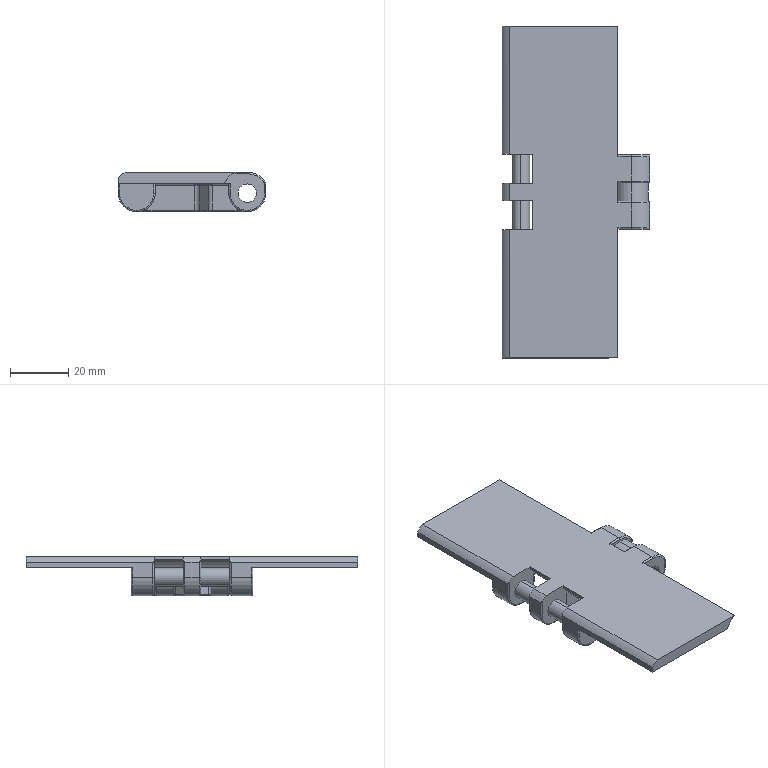Part | SolidWorks | features BaseBody 1 | 1 solid | 156 faces | box 50.9 x 114.3 x 13.6 mm | volume 23056 mm3 | cylinder 81 | plane 42 | spline 33 | commonest cylinder face diameters 1 x40 12.8 x13 4 x10 6.36 x4 16.473 x3 17.088 x3